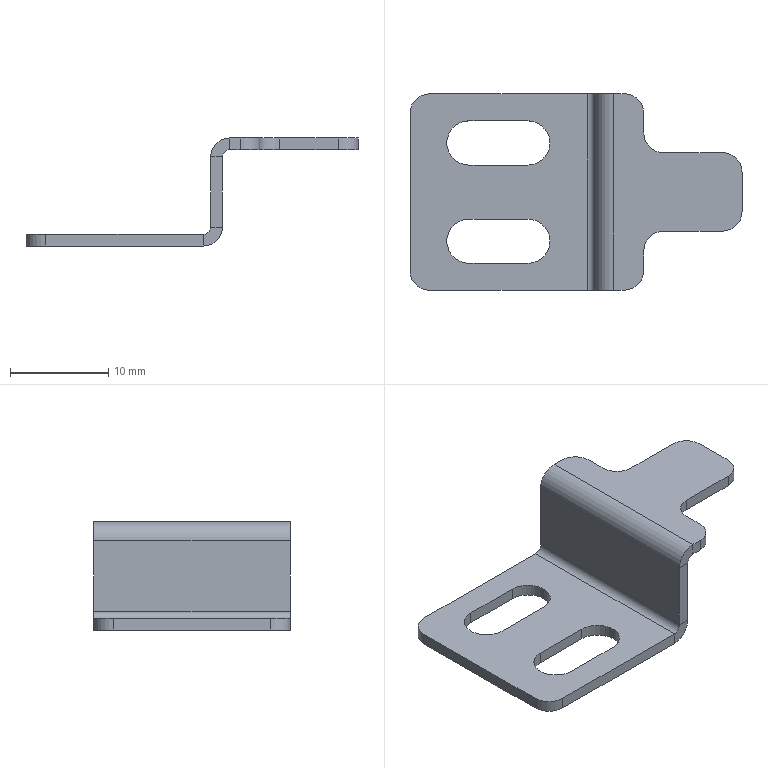Part | SolidWorks | features EdgeFlange 2, ICE 2, Fillet 1, FlatPattern 1, SMBaseFlange 1, SheetMetal 1 | 1 solid | 44 faces | box 33.8 x 20 x 11 mm | volume 767.773 mm3 | plane 26 | cylinder 18 | commonest cylinder face diameters 4 x8 4.5 x6 1.473 x2 3.873 x2
STEP:
#1=CARTESIAN_POINT('',(4.25,-5.,-1.2));
#2=VERTEX_POINT('',#1);
#3=CARTESIAN_POINT('',(2.,-2.75,-1.2));
#4=VERTEX_POINT('',#3);
#5=CARTESIAN_POINT('',(2.,-5.,-1.2));
#6=DIRECTION('',(0.,0.,1.));
#7=DIRECTION('',(-1.,0.,0.));
#8=AXIS2_PLACEMENT_3D('',#5,#6,#7);
#9=CIRCLE('',#8,2.25);
#10=EDGE_CURVE('',#2,#4,#9,.T.);
#11=ORIENTED_EDGE('',*,*,#10,.F.);
#12=CARTESIAN_POINT('',(4.25,-5.,0.));
#13=VERTEX_POINT('',#12);
#14=CARTESIAN_POINT('',(4.25,-5.,-1.2));
#15=DIRECTION('',(0.,0.,1.));
#16=VECTOR('',#15,1000.);
#17=LINE('',#14,#16);
#18=EDGE_CURVE('',#2,#13,#17,.T.);
#19=ORIENTED_EDGE('',*,*,#18,.T.);
#20=CARTESIAN_POINT('',(2.,-2.75,0.));
#21=VERTEX_POINT('',#20);
#22=CARTESIAN_POINT('',(2.,-5.,0.));
#23=DIRECTION('',(0.,0.,1.));
#24=DIRECTION('',(-1.,0.,0.));
#25=AXIS2_PLACEMENT_3D('',#22,#23,#24);
#26=CIRCLE('',#25,2.25);
#27=EDGE_CURVE('',#13,#21,#26,.T.);
#28=ORIENTED_EDGE('',*,*,#27,.T.);
#29=CARTESIAN_POINT('',(2.,-2.75,-1.2));
#30=DIRECTION('',(0.,0.,1.));
#31=VECTOR('',#30,1000.);
#32=LINE('',#29,#31);
#33=EDGE_CURVE('',#4,#21,#32,.T.);
#34=ORIENTED_EDGE('',*,*,#33,.F.);
#35=EDGE_LOOP('',(#11,#19,#28,#34));
#36=FACE_OUTER_BOUND('',#35,.T.);
#37=CARTESIAN_POINT('',(2.,-5.,-1.2));
#38=DIRECTION('',(0.,0.,1.));
#39=DIRECTION('',(1.,0.,0.));
#40=AXIS2_PLACEMENT_3D('',#37,#38,#39);
#41=CYLINDRICAL_SURFACE('',#40,2.25);
#42=ADVANCED_FACE('',(#36),#41,.F.);
#43=CARTESIAN_POINT('',(4.25,5.,-1.2));
#44=VERTEX_POINT('',#43);
#45=CARTESIAN_POINT('',(2.,7.25,-1.2));
#46=VERTEX_POINT('',#45);
#47=CARTESIAN_POINT('',(2.,5.,-1.2));
#48=DIRECTION('',(0.,0.,1.));
#49=DIRECTION('',(1.,0.,0.));
#50=AXIS2_PLACEMENT_3D('',#47,#48,#49);
#51=CIRCLE('',#50,2.25);
#52=EDGE_CURVE('',#44,#46,#51,.T.);
#53=ORIENTED_EDGE('',*,*,#52,.F.);
#54=CARTESIAN_POINT('',(4.25,5.,0.));
#55=VERTEX_POINT('',#54);
#56=CARTESIAN_POINT('',(4.25,5.,-1.2));
#57=DIRECTION('',(0.,0.,1.));
#58=VECTOR('',#57,1000.);
#59=LINE('',#56,#58);
#60=EDGE_CURVE('',#44,#55,#59,.T.);
#61=ORIENTED_EDGE('',*,*,#60,.T.);
#62=CARTESIAN_POINT('',(2.,7.25,0.));
#63=VERTEX_POINT('',#62);
#64=CARTESIAN_POINT('',(2.,5.,0.));
#65=DIRECTION('',(0.,0.,1.));
#66=DIRECTION('',(1.,0.,0.));
#67=AXIS2_PLACEMENT_3D('',#64,#65,#66);
#68=CIRCLE('',#67,2.25);
#69=EDGE_CURVE('',#55,#63,#68,.T.);
#70=ORIENTED_EDGE('',*,*,#69,.T.);
#71=CARTESIAN_POINT('',(2.,7.25,-1.2));
#72=DIRECTION('',(0.,0.,1.));
#73=VECTOR('',#72,1000.);
#74=LINE('',#71,#73);
#75=EDGE_CURVE('',#46,#63,#74,.T.);
#76=ORIENTED_EDGE('',*,*,#75,.F.);
#77=EDGE_LOOP('',(#53,#61,#70,#76));
#78=FACE_OUTER_BOUND('',#77,.T.);
#79=CARTESIAN_POINT('',(2.,5.,-1.2));
#80=DIRECTION('',(0.,0.,1.));
#81=DIRECTION('',(1.,0.,0.));
#82=AXIS2_PLACEMENT_3D('',#79,#80,#81);
#83=CYLINDRICAL_SURFACE('',#82,2.25);
#84=ADVANCED_FACE('',(#78),#83,.F.);
#85=CARTESIAN_POINT('',(10.,-10.,0.7366));
#86=VERTEX_POINT('',#85);
#87=CARTESIAN_POINT('',(10.,-10.,7.863));
#88=VERTEX_POINT('',#87);
#89=CARTESIAN_POINT('',(10.,-10.,9.8));
#90=DIRECTION('',(0.,0.,1.));
#91=VECTOR('',#90,1000.);
#92=LINE('',#89,#91);
#93=EDGE_CURVE('',#86,#88,#92,.T.);
#94=ORIENTED_EDGE('',*,*,#93,.T.);
#95=CARTESIAN_POINT('',(8.8,-10.,7.863));
#96=VERTEX_POINT('',#95);
#97=CARTESIAN_POINT('',(10.,-10.,7.863));
#98=DIRECTION('',(-1.,0.,0.));
#99=VECTOR('',#98,1000.);
#100=LINE('',#97,#99);
#101=EDGE_CURVE('',#88,#96,#100,.T.);
#102=ORIENTED_EDGE('',*,*,#101,.T.);
#103=CARTESIAN_POINT('',(8.8,-10.,0.7366));
#104=VERTEX_POINT('',#103);
#105=CARTESIAN_POINT('',(8.8,-10.,0.));
#106=DIRECTION('',(0.,0.,1.));
#107=VECTOR('',#106,1000.);
#108=LINE('',#105,#107);
#109=EDGE_CURVE('',#104,#96,#108,.T.);
#110=ORIENTED_EDGE('',*,*,#109,.F.);
#111=CARTESIAN_POINT('',(10.,-10.,0.7366));
#112=DIRECTION('',(1.,0.,0.));
#113=VECTOR('',#112,1000.);
#114=LINE('',#111,#113);
#115=EDGE_CURVE('',#104,#86,#114,.T.);
#116=ORIENTED_EDGE('',*,*,#115,.T.);
#117=EDGE_LOOP('',(#94,#102,#110,#116));
#118=FACE_OUTER_BOUND('',#117,.T.);
#119=CARTESIAN_POINT('',(10.,-10.,9.8));
#120=DIRECTION('',(0.,-1.,0.));
#121=DIRECTION('',(0.,0.,-1.));
#122=AXIS2_PLACEMENT_3D('',#119,#120,#121);
#123=PLANE('',#122);
#124=ADVANCED_FACE('',(#118),#123,.T.);
#125=CARTESIAN_POINT('',(10.,10.,7.863));
#126=VERTEX_POINT('',#125);
#127=CARTESIAN_POINT('',(10.,10.,0.7366));
#128=VERTEX_POINT('',#127);
#129=CARTESIAN_POINT('',(10.,10.,0.));
#130=DIRECTION('',(0.,0.,-1.));
#131=VECTOR('',#130,1000.);
#132=LINE('',#129,#131);
#133=EDGE_CURVE('',#126,#128,#132,.T.);
#134=ORIENTED_EDGE('',*,*,#133,.F.);
#135=CARTESIAN_POINT('',(10.,-10.,7.863));
#136=DIRECTION('',(0.,1.,0.));
#137=VECTOR('',#136,1000.);
#138=LINE('',#135,#137);
#139=EDGE_CURVE('',#88,#126,#138,.T.);
#140=ORIENTED_EDGE('',*,*,#139,.F.);
#141=ORIENTED_EDGE('',*,*,#93,.F.);
#142=CARTESIAN_POINT('',(10.,0.,0.7366));
#143=DIRECTION('',(0.,1.,0.));
#144=VECTOR('',#143,1000.);
#145=LINE('',#142,#144);
#146=EDGE_CURVE('',#86,#128,#145,.T.);
#147=ORIENTED_EDGE('',*,*,#146,.T.);
#148=EDGE_LOOP('',(#134,#140,#141,#147));
#149=FACE_OUTER_BOUND('',#148,.T.);
#150=CARTESIAN_POINT('',(10.,0.,0.));
#151=DIRECTION('',(1.,0.,0.));
#152=DIRECTION('',(0.,0.,-1.));
#153=AXIS2_PLACEMENT_3D('',#150,#151,#152);
#154=PLANE('',#153);
#155=ADVANCED_FACE('',(#149),#154,.T.);
#156=CARTESIAN_POINT('',(8.8,10.,7.863));
#157=VERTEX_POINT('',#156);
#158=CARTESIAN_POINT('',(8.8,-10.,7.863));
#159=DIRECTION('',(0.,1.,0.));
#160=VECTOR('',#159,1000.);
#161=LINE('',#158,#160);
#162=EDGE_CURVE('',#96,#157,#161,.T.);
#163=ORIENTED_EDGE('',*,*,#162,.T.);
#164=CARTESIAN_POINT('',(8.8,10.,0.7366));
#165=VERTEX_POINT('',#164);
#166=CARTESIAN_POINT('',(8.8,10.,0.));
#167=DIRECTION('',(0.,0.,-1.));
#168=VECTOR('',#167,1000.);
#169=LINE('',#166,#168);
#170=EDGE_CURVE('',#157,#165,#169,.T.);
#171=ORIENTED_EDGE('',*,*,#170,.T.);
#172=CARTESIAN_POINT('',(8.8,-10.,0.7366));
#173=DIRECTION('',(0.,1.,0.));
#174=VECTOR('',#173,1000.);
#175=LINE('',#172,#174);
#176=EDGE_CURVE('',#104,#165,#175,.T.);
#177=ORIENTED_EDGE('',*,*,#176,.F.);
#178=ORIENTED_EDGE('',*,*,#109,.T.);
#179=EDGE_LOOP('',(#163,#171,#177,#178));
#180=FACE_OUTER_BOUND('',#179,.T.);
#181=CARTESIAN_POINT('',(8.8,0.,0.));
#182=DIRECTION('',(1.,0.,0.));
#183=DIRECTION('',(0.,0.,-1.));
#184=AXIS2_PLACEMENT_3D('',#181,#182,#183);
#185=PLANE('',#184);
#186=ADVANCED_FACE('',(#180),#185,.F.);
#187=CARTESIAN_POINT('',(8.063,10.,-1.2));
#188=VERTEX_POINT('',#187);
#189=CARTESIAN_POINT('',(-8.,10.,-1.2));
#190=VERTEX_POINT('',#189);
#191=CARTESIAN_POINT('',(-10.,10.,-1.2));
#192=DIRECTION('',(-1.,0.,0.));
#193=VECTOR('',#192,1000.);
#194=LINE('',#191,#193);
#195=EDGE_CURVE('',#188,#190,#194,.T.);
#196=ORIENTED_EDGE('',*,*,#195,.T.);
#197=CARTESIAN_POINT('',(-8.,10.,0.));
#198=VERTEX_POINT('',#197);
#199=CARTESIAN_POINT('',(-8.,10.,-1.2));
#200=DIRECTION('',(0.,0.,1.));
#201=VECTOR('',#200,1000.);
#202=LINE('',#199,#201);
#203=EDGE_CURVE('',#190,#198,#202,.T.);
#204=ORIENTED_EDGE('',*,*,#203,.T.);
#205=CARTESIAN_POINT('',(8.063,10.,0.));
#206=VERTEX_POINT('',#205);
#207=CARTESIAN_POINT('',(-10.,10.,0.));
#208=DIRECTION('',(-1.,0.,0.));
#209=VECTOR('',#208,1000.);
#210=LINE('',#207,#209);
#211=EDGE_CURVE('',#206,#198,#210,.T.);
#212=ORIENTED_EDGE('',*,*,#211,.F.);
#213=CARTESIAN_POINT('',(8.063,10.,0.));
#214=DIRECTION('',(0.,0.,-1.));
#215=VECTOR('',#214,1000.);
#216=LINE('',#213,#215);
#217=EDGE_CURVE('',#206,#188,#216,.T.);
#218=ORIENTED_EDGE('',*,*,#217,.T.);
#219=EDGE_LOOP('',(#196,#204,#212,#218));
#220=FACE_OUTER_BOUND('',#219,.T.);
#221=CARTESIAN_POINT('',(-10.,10.,-1.2));
#222=DIRECTION('',(0.,1.,0.));
#223=DIRECTION('',(0.,0.,1.));
#224=AXIS2_PLACEMENT_3D('',#221,#222,#223);
#225=PLANE('',#224);
#226=ADVANCED_FACE('',(#220),#225,.T.);
#227=CARTESIAN_POINT('',(-4.,-2.75,-1.2));
#228=VERTEX_POINT('',#227);
#229=CARTESIAN_POINT('',(-4.,-7.25,-1.2));
#230=VERTEX_POINT('',#229);
#231=CARTESIAN_POINT('',(-4.,-5.,-1.2));
#232=DIRECTION('',(0.,0.,1.));
#233=DIRECTION('',(-1.,0.,0.));
#234=AXIS2_PLACEMENT_3D('',#231,#232,#233);
#235=CIRCLE('',#234,2.25);
#236=EDGE_CURVE('',#228,#230,#235,.T.);
#237=ORIENTED_EDGE('',*,*,#236,.T.);
#238=CARTESIAN_POINT('',(2.,-7.25,-1.2));
#239=VERTEX_POINT('',#238);
#240=CARTESIAN_POINT('',(-4.,-7.25,-1.2));
#241=DIRECTION('',(1.,0.,0.));
#242=VECTOR('',#241,1000.);
#243=LINE('',#240,#242);
#244=EDGE_CURVE('',#230,#239,#243,.T.);
#245=ORIENTED_EDGE('',*,*,#244,.T.);
#246=CARTESIAN_POINT('',(2.,-5.,-1.2));
#247=DIRECTION('',(0.,0.,1.));
#248=DIRECTION('',(-1.,0.,0.));
#249=AXIS2_PLACEMENT_3D('',#246,#247,#248);
#250=CIRCLE('',#249,2.25);
#251=EDGE_CURVE('',#239,#2,#250,.T.);
#252=ORIENTED_EDGE('',*,*,#251,.T.);
#253=ORIENTED_EDGE('',*,*,#10,.T.);
#254=CARTESIAN_POINT('',(-4.,-2.75,-1.2));
#255=DIRECTION('',(-1.,0.,0.));
#256=VECTOR('',#255,1000.);
#257=LINE('',#254,#256);
#258=EDGE_CURVE('',#4,#228,#257,.T.);
#259=ORIENTED_EDGE('',*,*,#258,.T.);
#260=EDGE_LOOP('',(#237,#245,#252,#253,#259));
#261=FACE_BOUND('',#260,.T.);
#262=CARTESIAN_POINT('',(-4.,7.25,-1.2));
#263=VERTEX_POINT('',#262);
#264=CARTESIAN_POINT('',(-4.,2.75,-1.2));
#265=VERTEX_POINT('',#264);
#266=CARTESIAN_POINT('',(-4.,5.,-1.2));
#267=DIRECTION('',(0.,0.,1.));
#268=DIRECTION('',(1.,0.,0.));
#269=AXIS2_PLACEMENT_3D('',#266,#267,#268);
#270=CIRCLE('',#269,2.25);
#271=EDGE_CURVE('',#263,#265,#270,.T.);
#272=ORIENTED_EDGE('',*,*,#271,.T.);
#273=CARTESIAN_POINT('',(2.,2.75,-1.2));
#274=VERTEX_POINT('',#273);
#275=CARTESIAN_POINT('',(-4.,2.75,-1.2));
#276=DIRECTION('',(1.,0.,0.));
#277=VECTOR('',#276,1000.);
#278=LINE('',#275,#277);
#279=EDGE_CURVE('',#265,#274,#278,.T.);
#280=ORIENTED_EDGE('',*,*,#279,.T.);
#281=CARTESIAN_POINT('',(2.,5.,-1.2));
#282=DIRECTION('',(0.,0.,1.));
#283=DIRECTION('',(1.,0.,0.));
#284=AXIS2_PLACEMENT_3D('',#281,#282,#283);
#285=CIRCLE('',#284,2.25);
#286=EDGE_CURVE('',#274,#44,#285,.T.);
#287=ORIENTED_EDGE('',*,*,#286,.T.);
#288=ORIENTED_EDGE('',*,*,#52,.T.);
#289=CARTESIAN_POINT('',(-4.,7.25,-1.2));
#290=DIRECTION('',(-1.,0.,0.));
#291=VECTOR('',#290,1000.);
#292=LINE('',#289,#291);
#293=EDGE_CURVE('',#46,#263,#292,.T.);
#294=ORIENTED_EDGE('',*,*,#293,.T.);
#295=EDGE_LOOP('',(#272,#280,#287,#288,#294));
#296=FACE_BOUND('',#295,.T.);
#297=CARTESIAN_POINT('',(-8.,-10.,-1.2));
#298=VERTEX_POINT('',#297);
#299=CARTESIAN_POINT('',(8.063,-10.,-1.2));
#300=VERTEX_POINT('',#299);
#301=CARTESIAN_POINT('',(-10.,-10.,-1.2));
#302=DIRECTION('',(1.,0.,0.));
#303=VECTOR('',#302,1000.);
#304=LINE('',#301,#303);
#305=EDGE_CURVE('',#298,#300,#304,.T.);
#306=ORIENTED_EDGE('',*,*,#305,.F.);
#307=CARTESIAN_POINT('',(-10.,-8.,-1.2));
#308=VERTEX_POINT('',#307);
#309=CARTESIAN_POINT('',(-8.,-8.,-1.2));
#310=DIRECTION('',(0.,0.,-1.));
#311=DIRECTION('',(-1.,0.,0.));
#312=AXIS2_PLACEMENT_3D('',#309,#310,#311);
#313=CIRCLE('',#312,2.);
#314=EDGE_CURVE('',#298,#308,#313,.T.);
#315=ORIENTED_EDGE('',*,*,#314,.T.);
#316=CARTESIAN_POINT('',(-10.,8.,-1.2));
#317=VERTEX_POINT('',#316);
#318=CARTESIAN_POINT('',(-10.,-10.,-1.2));
#319=DIRECTION('',(0.,-1.,0.));
#320=VECTOR('',#319,1000.);
#321=LINE('',#318,#320);
#322=EDGE_CURVE('',#317,#308,#321,.T.);
#323=ORIENTED_EDGE('',*,*,#322,.F.);
#324=CARTESIAN_POINT('',(-8.,8.,-1.2));
#325=DIRECTION('',(0.,0.,-1.));
#326=DIRECTION('',(-1.,0.,0.));
#327=AXIS2_PLACEMENT_3D('',#324,#325,#326);
#328=CIRCLE('',#327,2.);
#329=EDGE_CURVE('',#317,#190,#328,.T.);
#330=ORIENTED_EDGE('',*,*,#329,.T.);
#331=ORIENTED_EDGE('',*,*,#195,.F.);
#332=CARTESIAN_POINT('',(8.063,10.,-1.2));
#333=DIRECTION('',(0.,-1.,0.));
#334=VECTOR('',#333,1000.);
#335=LINE('',#332,#334);
#336=EDGE_CURVE('',#188,#300,#335,.T.);
#337=ORIENTED_EDGE('',*,*,#336,.T.);
#338=EDGE_LOOP('',(#306,#315,#323,#330,#331,#337));
#339=FACE_OUTER_BOUND('',#338,.T.);
#340=CARTESIAN_POINT('',(0.,0.,-1.2));
#341=DIRECTION('',(0.,0.,-1.));
#342=DIRECTION('',(-1.,0.,0.));
#343=AXIS2_PLACEMENT_3D('',#340,#341,#342);
#344=PLANE('',#343);
#345=ADVANCED_FACE('',(#261,#296,#339),#344,.T.);
#346=CARTESIAN_POINT('',(-4.,-7.25,0.));
#347=VERTEX_POINT('',#346);
#348=CARTESIAN_POINT('',(2.,-7.25,0.));
#349=VERTEX_POINT('',#348);
#350=CARTESIAN_POINT('',(-4.,-7.25,0.));
#351=DIRECTION('',(1.,0.,0.));
#352=VECTOR('',#351,1000.);
#353=LINE('',#350,#352);
#354=EDGE_CURVE('',#347,#349,#353,.T.);
#355=ORIENTED_EDGE('',*,*,#354,.F.);
#356=CARTESIAN_POINT('',(-4.,-2.75,0.));
#357=VERTEX_POINT('',#356);
#358=CARTESIAN_POINT('',(-4.,-5.,0.));
#359=DIRECTION('',(0.,0.,1.));
#360=DIRECTION('',(-1.,0.,0.));
#361=AXIS2_PLACEMENT_3D('',#358,#359,#360);
#362=CIRCLE('',#361,2.25);
#363=EDGE_CURVE('',#357,#347,#362,.T.);
#364=ORIENTED_EDGE('',*,*,#363,.F.);
#365=CARTESIAN_POINT('',(-4.,-2.75,0.));
#366=DIRECTION('',(-1.,0.,0.));
#367=VECTOR('',#366,1000.);
#368=LINE('',#365,#367);
#369=EDGE_CURVE('',#21,#357,#368,.T.);
#370=ORIENTED_EDGE('',*,*,#369,.F.);
#371=ORIENTED_EDGE('',*,*,#27,.F.);
#372=CARTESIAN_POINT('',(2.,-5.,0.));
#373=DIRECTION('',(0.,0.,1.));
#374=DIRECTION('',(-1.,0.,0.));
#375=AXIS2_PLACEMENT_3D('',#372,#373,#374);
#376=CIRCLE('',#375,2.25);
#377=EDGE_CURVE('',#349,#13,#376,.T.);
#378=ORIENTED_EDGE('',*,*,#377,.F.);
#379=EDGE_LOOP('',(#355,#364,#370,#371,#378));
#380=FACE_BOUND('',#379,.T.);
#381=CARTESIAN_POINT('',(-4.,2.75,0.));
#382=VERTEX_POINT('',#381);
#383=CARTESIAN_POINT('',(2.,2.75,0.));
#384=VERTEX_POINT('',#383);
#385=CARTESIAN_POINT('',(-4.,2.75,0.));
#386=DIRECTION('',(1.,0.,0.));
#387=VECTOR('',#386,1000.);
#388=LINE('',#385,#387);
#389=EDGE_CURVE('',#382,#384,#388,.T.);
#390=ORIENTED_EDGE('',*,*,#389,.F.);
#391=CARTESIAN_POINT('',(-4.,7.25,0.));
#392=VERTEX_POINT('',#391);
#393=CARTESIAN_POINT('',(-4.,5.,0.));
#394=DIRECTION('',(0.,0.,1.));
#395=DIRECTION('',(1.,0.,0.));
#396=AXIS2_PLACEMENT_3D('',#393,#394,#395);
#397=CIRCLE('',#396,2.25);
#398=EDGE_CURVE('',#392,#382,#397,.T.);
#399=ORIENTED_EDGE('',*,*,#398,.F.);
#400=CARTESIAN_POINT('',(-4.,7.25,0.));
#401=DIRECTION('',(-1.,0.,0.));
#402=VECTOR('',#401,1000.);
#403=LINE('',#400,#402);
#404=EDGE_CURVE('',#63,#392,#403,.T.);
#405=ORIENTED_EDGE('',*,*,#404,.F.);
#406=ORIENTED_EDGE('',*,*,#69,.F.);
#407=CARTESIAN_POINT('',(2.,5.,0.));
#408=DIRECTION('',(0.,0.,1.));
#409=DIRECTION('',(1.,0.,0.));
#410=AXIS2_PLACEMENT_3D('',#407,#408,#409);
#411=CIRCLE('',#410,2.25);
#412=EDGE_CURVE('',#384,#55,#411,.T.);
#413=ORIENTED_EDGE('',*,*,#412,.F.);
#414=EDGE_LOOP('',(#390,#399,#405,#406,#413));
#415=FACE_BOUND('',#414,.T.);
#416=CARTESIAN_POINT('',(-10.,8.,0.));
#417=VERTEX_POINT('',#416);
#418=CARTESIAN_POINT('',(-10.,-8.,0.));
#419=VERTEX_POINT('',#418);
#420=CARTESIAN_POINT('',(-10.,-10.,0.));
#421=DIRECTION('',(0.,-1.,0.));
#422=VECTOR('',#421,1000.);
#423=LINE('',#420,#422);
#424=EDGE_CURVE('',#417,#419,#423,.T.);
#425=ORIENTED_EDGE('',*,*,#424,.T.);
#426=CARTESIAN_POINT('',(-8.,-10.,0.));
#427=VERTEX_POINT('',#426);
#428=CARTESIAN_POINT('',(-8.,-8.,0.));
#429=DIRECTION('',(0.,0.,1.));
#430=DIRECTION('',(-1.,0.,0.));
#431=AXIS2_PLACEMENT_3D('',#428,#429,#430);
#432=CIRCLE('',#431,2.);
#433=EDGE_CURVE('',#419,#427,#432,.T.);
#434=ORIENTED_EDGE('',*,*,#433,.T.);
#435=CARTESIAN_POINT('',(8.063,-10.,0.));
#436=VERTEX_POINT('',#435);
#437=CARTESIAN_POINT('',(-10.,-10.,0.));
#438=DIRECTION('',(1.,0.,0.));
#439=VECTOR('',#438,1000.);
#440=LINE('',#437,#439);
#441=EDGE_CURVE('',#427,#436,#440,.T.);
#442=ORIENTED_EDGE('',*,*,#441,.T.);
#443=CARTESIAN_POINT('',(8.063,10.,0.));
#444=DIRECTION('',(0.,-1.,0.));
#445=VECTOR('',#444,1000.);
#446=LINE('',#443,#445);
#447=EDGE_CURVE('',#206,#436,#446,.T.);
#448=ORIENTED_EDGE('',*,*,#447,.F.);
#449=ORIENTED_EDGE('',*,*,#211,.T.);
#450=CARTESIAN_POINT('',(-8.,8.,0.));
#451=DIRECTION('',(0.,0.,1.));
#452=DIRECTION('',(-1.,0.,0.));
#453=AXIS2_PLACEMENT_3D('',#450,#451,#452);
#454=CIRCLE('',#453,2.);
#455=EDGE_CURVE('',#198,#417,#454,.T.);
#456=ORIENTED_EDGE('',*,*,#455,.T.);
#457=EDGE_LOOP('',(#425,#434,#442,#448,#449,#456));
#458=FACE_OUTER_BOUND('',#457,.T.);
#459=CARTESIAN_POINT('',(0.,0.,0.));
#460=DIRECTION('',(0.,0.,-1.));
#461=DIRECTION('',(-1.,0.,0.));
#462=AXIS2_PLACEMENT_3D('',#459,#460,#461);
#463=PLANE('',#462);
#464=ADVANCED_FACE('',(#380,#415,#458),#463,.F.);
#465=ORIENTED_EDGE('',*,*,#441,.F.);
#466=CARTESIAN_POINT('',(-8.,-10.,-1.2));
#467=DIRECTION('',(0.,0.,-1.));
#468=VECTOR('',#467,1000.);
#469=LINE('',#466,#468);
#470=EDGE_CURVE('',#427,#298,#469,.T.);
#471=ORIENTED_EDGE('',*,*,#470,.T.);
#472=ORIENTED_EDGE('',*,*,#305,.T.);
#473=CARTESIAN_POINT('',(8.063,-10.,0.));
#474=DIRECTION('',(0.,0.,-1.));
#475=VECTOR('',#474,1000.);
#476=LINE('',#473,#475);
#477=EDGE_CURVE('',#436,#300,#476,.T.);
#478=ORIENTED_EDGE('',*,*,#477,.F.);
#479=EDGE_LOOP('',(#465,#471,#472,#478));
#480=FACE_OUTER_BOUND('',#479,.T.);
#481=CARTESIAN_POINT('',(-10.,-10.,-1.2));
#482=DIRECTION('',(0.,-1.,0.));
#483=DIRECTION('',(0.,0.,-1.));
#484=AXIS2_PLACEMENT_3D('',#481,#482,#483);
#485=PLANE('',#484);
#486=ADVANCED_FACE('',(#480),#485,.T.);
#487=ORIENTED_EDGE('',*,*,#322,.T.);
#488=CARTESIAN_POINT('',(-10.,-8.,-1.2));
#489=DIRECTION('',(0.,0.,1.));
#490=VECTOR('',#489,1000.);
#491=LINE('',#488,#490);
#492=EDGE_CURVE('',#308,#419,#491,.T.);
#493=ORIENTED_EDGE('',*,*,#492,.T.);
#494=ORIENTED_EDGE('',*,*,#424,.F.);
#495=CARTESIAN_POINT('',(-10.,8.,-1.2));
#496=DIRECTION('',(0.,0.,-1.));
#497=VECTOR('',#496,1000.);
#498=LINE('',#495,#497);
#499=EDGE_CURVE('',#417,#317,#498,.T.);
#500=ORIENTED_EDGE('',*,*,#499,.T.);
#501=EDGE_LOOP('',(#487,#493,#494,#500));
#502=FACE_OUTER_BOUND('',#501,.T.);
#503=CARTESIAN_POINT('',(-10.,-10.,-1.2));
#504=DIRECTION('',(-1.,0.,0.));
#505=DIRECTION('',(0.,0.,1.));
#506=AXIS2_PLACEMENT_3D('',#503,#504,#505);
#507=PLANE('',#506);
#508=ADVANCED_FACE('',(#502),#507,.T.);
#509=ORIENTED_EDGE('',*,*,#115,.F.);
#510=CARTESIAN_POINT('',(8.063,-10.,0.7366));
#511=DIRECTION('',(0.,-1.,0.));
#512=DIRECTION('',(0.,0.,1.));
#513=AXIS2_PLACEMENT_3D('',#510,#511,#512);
#514=CIRCLE('',#513,0.7366);
#515=EDGE_CURVE('',#436,#104,#514,.T.);
#516=ORIENTED_EDGE('',*,*,#515,.F.);
#517=ORIENTED_EDGE('',*,*,#477,.T.);
#518=CARTESIAN_POINT('',(8.063,-10.,0.7366));
#519=DIRECTION('',(0.,-1.,0.));
#520=DIRECTION('',(0.,0.,1.));
#521=AXIS2_PLACEMENT_3D('',#518,#519,#520);
#522=CIRCLE('',#521,1.937);
#523=EDGE_CURVE('',#300,#86,#522,.T.);
#524=ORIENTED_EDGE('',*,*,#523,.T.);
#525=EDGE_LOOP('',(#509,#516,#517,#524));
#526=FACE_OUTER_BOUND('',#525,.T.);
#527=CARTESIAN_POINT('',(8.063,-10.,0.7366));
#528=DIRECTION('',(0.,-1.,0.));
#529=DIRECTION('',(0.,0.,-1.));
#530=AXIS2_PLACEMENT_3D('',#527,#528,#529);
#531=PLANE('',#530);
#532=ADVANCED_FACE('',(#526),#531,.T.);
#533=CARTESIAN_POINT('',(8.063,10.,0.7366));
#534=DIRECTION('',(0.,1.,0.));
#535=DIRECTION('',(0.,0.,1.));
#536=AXIS2_PLACEMENT_3D('',#533,#534,#535);
#537=CIRCLE('',#536,0.7366);
#538=EDGE_CURVE('',#165,#206,#537,.T.);
#539=ORIENTED_EDGE('',*,*,#538,.F.);
#540=CARTESIAN_POINT('',(8.8,10.,0.7366));
#541=DIRECTION('',(1.,0.,0.));
#542=VECTOR('',#541,1000.);
#543=LINE('',#540,#542);
#544=EDGE_CURVE('',#165,#128,#543,.T.);
#545=ORIENTED_EDGE('',*,*,#544,.T.);
#546=CARTESIAN_POINT('',(8.063,10.,0.7366));
#547=DIRECTION('',(0.,1.,0.));
#548=DIRECTION('',(0.,0.,1.));
#549=AXIS2_PLACEMENT_3D('',#546,#547,#548);
#550=CIRCLE('',#549,1.937);
#551=EDGE_CURVE('',#128,#188,#550,.T.);
#552=ORIENTED_EDGE('',*,*,#551,.T.);
#553=ORIENTED_EDGE('',*,*,#217,.F.);
#554=EDGE_LOOP('',(#539,#545,#552,#553));
#555=FACE_OUTER_BOUND('',#554,.T.);
#556=CARTESIAN_POINT('',(8.063,10.,0.7366));
#557=DIRECTION('',(0.,-1.,0.));
#558=DIRECTION('',(0.,0.,-1.));
#559=AXIS2_PLACEMENT_3D('',#556,#557,#558);
#560=PLANE('',#559);
#561=ADVANCED_FACE('',(#555),#560,.F.);
#562=ORIENTED_EDGE('',*,*,#336,.F.);
#563=ORIENTED_EDGE('',*,*,#551,.F.);
#564=ORIENTED_EDGE('',*,*,#146,.F.);
#565=ORIENTED_EDGE('',*,*,#523,.F.);
#566=EDGE_LOOP('',(#562,#563,#564,#565));
#567=FACE_OUTER_BOUND('',#566,.T.);
#568=CARTESIAN_POINT('',(8.063,10.,0.7366));
#569=DIRECTION('',(0.,1.,0.));
#570=DIRECTION('',(1.,0.,0.));
#571=AXIS2_PLACEMENT_3D('',#568,#569,#570);
#572=CYLINDRICAL_SURFACE('',#571,1.937);
#573=ADVANCED_FACE('',(#567),#572,.T.);
#574=ORIENTED_EDGE('',*,*,#447,.T.);
#575=ORIENTED_EDGE('',*,*,#515,.T.);
#576=ORIENTED_EDGE('',*,*,#176,.T.);
#577=ORIENTED_EDGE('',*,*,#538,.T.);
#578=EDGE_LOOP('',(#574,#575,#576,#577));
#579=FACE_OUTER_BOUND('',#578,.T.);
#580=CARTESIAN_POINT('',(8.063,10.,0.7366));
#581=DIRECTION('',(0.,1.,0.));
#582=DIRECTION('',(1.,0.,0.));
#583=AXIS2_PLACEMENT_3D('',#580,#581,#582);
#584=CYLINDRICAL_SURFACE('',#583,0.7366);
#585=ADVANCED_FACE('',(#579),#584,.F.);
#586=CARTESIAN_POINT('',(10.,10.,7.863));
#587=DIRECTION('',(-1.,0.,0.));
#588=VECTOR('',#587,1000.);
#589=LINE('',#586,#588);
#590=EDGE_CURVE('',#126,#157,#589,.T.);
#591=ORIENTED_EDGE('',*,*,#590,.F.);
#592=ORIENTED_EDGE('',*,*,#133,.T.);
#593=ORIENTED_EDGE('',*,*,#544,.F.);
#594=ORIENTED_EDGE('',*,*,#170,.F.);
#595=EDGE_LOOP('',(#591,#592,#593,#594));
#596=FACE_OUTER_BOUND('',#595,.T.);
#597=CARTESIAN_POINT('',(10.,10.,0.));
#598=DIRECTION('',(0.,1.,0.));
#599=DIRECTION('',(0.,0.,1.));
#600=AXIS2_PLACEMENT_3D('',#597,#598,#599);
#601=PLANE('',#600);
#602=ADVANCED_FACE('',(#596),#601,.T.);
#603=CARTESIAN_POINT('',(10.737,10.,8.6));
#604=VERTEX_POINT('',#603);
#605=CARTESIAN_POINT('',(10.737,10.,9.8));
#606=VERTEX_POINT('',#605);
#607=CARTESIAN_POINT('',(10.737,10.,9.8));
#608=DIRECTION('',(0.,0.,1.));
#609=VECTOR('',#608,1000.);
#610=LINE('',#607,#609);
#611=EDGE_CURVE('',#604,#606,#610,.T.);
#612=ORIENTED_EDGE('',*,*,#611,.F.);
#613=CARTESIAN_POINT('',(10.737,10.,7.863));
#614=DIRECTION('',(0.,1.,0.));
#615=DIRECTION('',(0.,0.,-1.));
#616=AXIS2_PLACEMENT_3D('',#613,#614,#615);
#617=CIRCLE('',#616,0.7366);
#618=EDGE_CURVE('',#126,#604,#617,.T.);
#619=ORIENTED_EDGE('',*,*,#618,.F.);
#620=ORIENTED_EDGE('',*,*,#590,.T.);
#621=CARTESIAN_POINT('',(10.737,10.,7.863));
#622=DIRECTION('',(0.,1.,0.));
#623=DIRECTION('',(0.,0.,-1.));
#624=AXIS2_PLACEMENT_3D('',#621,#622,#623);
#625=CIRCLE('',#624,1.937);
#626=EDGE_CURVE('',#157,#606,#625,.T.);
#627=ORIENTED_EDGE('',*,*,#626,.T.);
#628=EDGE_LOOP('',(#612,#619,#620,#627));
#629=FACE_OUTER_BOUND('',#628,.T.);
#630=CARTESIAN_POINT('',(10.737,10.,7.863));
#631=DIRECTION('',(0.,1.,0.));
#632=DIRECTION('',(0.,0.,1.));
#633=AXIS2_PLACEMENT_3D('',#630,#631,#632);
#634=PLANE('',#633);
#635=ADVANCED_FACE('',(#629),#634,.T.);
#636=CARTESIAN_POINT('',(10.737,-10.,8.6));
#637=VERTEX_POINT('',#636);
#638=CARTESIAN_POINT('',(10.737,-10.,7.863));
#639=DIRECTION('',(0.,-1.,0.));
#640=DIRECTION('',(0.,0.,-1.));
#641=AXIS2_PLACEMENT_3D('',#638,#639,#640);
#642=CIRCLE('',#641,0.7366);
#643=EDGE_CURVE('',#637,#88,#642,.T.);
#644=ORIENTED_EDGE('',*,*,#643,.F.);
#645=CARTESIAN_POINT('',(10.737,-10.,9.8));
#646=VERTEX_POINT('',#645);
#647=CARTESIAN_POINT('',(10.737,-10.,8.6));
#648=DIRECTION('',(0.,0.,1.));
#649=VECTOR('',#648,1000.);
#650=LINE('',#647,#649);
#651=EDGE_CURVE('',#637,#646,#650,.T.);
#652=ORIENTED_EDGE('',*,*,#651,.T.);
#653=CARTESIAN_POINT('',(10.737,-10.,7.863));
#654=DIRECTION('',(0.,-1.,0.));
#655=DIRECTION('',(0.,0.,-1.));
#656=AXIS2_PLACEMENT_3D('',#653,#654,#655);
#657=CIRCLE('',#656,1.937);
#658=EDGE_CURVE('',#646,#96,#657,.T.);
#659=ORIENTED_EDGE('',*,*,#658,.T.);
#660=ORIENTED_EDGE('',*,*,#101,.F.);
#661=EDGE_LOOP('',(#644,#652,#659,#660));
#662=FACE_OUTER_BOUND('',#661,.T.);
#663=CARTESIAN_POINT('',(10.737,-10.,7.863));
#664=DIRECTION('',(0.,1.,0.));
#665=DIRECTION('',(0.,0.,1.));
#666=AXIS2_PLACEMENT_3D('',#663,#664,#665);
#667=PLANE('',#666);
#668=ADVANCED_FACE('',(#662),#667,.F.);
#669=ORIENTED_EDGE('',*,*,#162,.F.);
#670=ORIENTED_EDGE('',*,*,#658,.F.);
#671=CARTESIAN_POINT('',(10.737,0.,9.8));
#672=DIRECTION('',(0.,-1.,0.));
#673=VECTOR('',#672,1000.);
#674=LINE('',#671,#673);
#675=EDGE_CURVE('',#606,#646,#674,.T.);
#676=ORIENTED_EDGE('',*,*,#675,.F.);
#677=ORIENTED_EDGE('',*,*,#626,.F.);
#678=EDGE_LOOP('',(#669,#670,#676,#677));
#679=FACE_OUTER_BOUND('',#678,.T.);
#680=CARTESIAN_POINT('',(10.737,-10.,7.863));
#681=DIRECTION('',(0.,-1.,0.));
#682=DIRECTION('',(0.,0.,1.));
#683=AXIS2_PLACEMENT_3D('',#680,#681,#682);
#684=CYLINDRICAL_SURFACE('',#683,1.937);
#685=ADVANCED_FACE('',(#679),#684,.T.);
#686=ORIENTED_EDGE('',*,*,#139,.T.);
#687=ORIENTED_EDGE('',*,*,#618,.T.);
#688=CARTESIAN_POINT('',(10.737,10.,8.6));
#689=DIRECTION('',(0.,-1.,0.));
#690=VECTOR('',#689,1000.);
#691=LINE('',#688,#690);
#692=EDGE_CURVE('',#604,#637,#691,.T.);
#693=ORIENTED_EDGE('',*,*,#692,.T.);
#694=ORIENTED_EDGE('',*,*,#643,.T.);
#695=EDGE_LOOP('',(#686,#687,#693,#694));
#696=FACE_OUTER_BOUND('',#695,.T.);
#697=CARTESIAN_POINT('',(10.737,-10.,7.863));
#698=DIRECTION('',(0.,-1.,0.));
#699=DIRECTION('',(0.,0.,1.));
#700=AXIS2_PLACEMENT_3D('',#697,#698,#699);
#701=CYLINDRICAL_SURFACE('',#700,0.7366);
#702=ADVANCED_FACE('',(#696),#701,.F.);
#703=CARTESIAN_POINT('',(11.8,-10.,8.6));
#704=VERTEX_POINT('',#703);
#705=CARTESIAN_POINT('',(0.,-10.,8.6));
#706=DIRECTION('',(-1.,0.,0.));
#707=VECTOR('',#706,1000.);
#708=LINE('',#705,#707);
#709=EDGE_CURVE('',#704,#637,#708,.T.);
#710=ORIENTED_EDGE('',*,*,#709,.F.);
#711=CARTESIAN_POINT('',(11.8,-10.,9.8));
#712=VERTEX_POINT('',#711);
#713=CARTESIAN_POINT('',(11.8,-10.,9.8));
#714=DIRECTION('',(0.,0.,1.));
#715=VECTOR('',#714,1000.);
#716=LINE('',#713,#715);
#717=EDGE_CURVE('',#704,#712,#716,.T.);
#718=ORIENTED_EDGE('',*,*,#717,.T.);
#719=CARTESIAN_POINT('',(10.,-10.,9.8));
#720=DIRECTION('',(-1.,0.,0.));
#721=VECTOR('',#720,1000.);
#722=LINE('',#719,#721);
#723=EDGE_CURVE('',#712,#646,#722,.T.);
#724=ORIENTED_EDGE('',*,*,#723,.T.);
#725=ORIENTED_EDGE('',*,*,#651,.F.);
#726=EDGE_LOOP('',(#710,#718,#724,#725));
#727=FACE_OUTER_BOUND('',#726,.T.);
#728=CARTESIAN_POINT('',(10.,-10.,9.8));
#729=DIRECTION('',(0.,-1.,0.));
#730=DIRECTION('',(0.,0.,-1.));
#731=AXIS2_PLACEMENT_3D('',#728,#729,#730);
#732=PLANE('',#731);
#733=ADVANCED_FACE('',(#727),#732,.T.);
#734=CARTESIAN_POINT('',(11.8,10.,9.8));
#735=VERTEX_POINT('',#734);
#736=CARTESIAN_POINT('',(23.8,10.,9.8));
#737=DIRECTION('',(1.,0.,0.));
#738=VECTOR('',#737,1000.);
#739=LINE('',#736,#738);
#740=EDGE_CURVE('',#606,#735,#739,.T.);
#741=ORIENTED_EDGE('',*,*,#740,.T.);
#742=CARTESIAN_POINT('',(11.8,10.,8.6));
#743=VERTEX_POINT('',#742);
#744=CARTESIAN_POINT('',(11.8,10.,8.6));
#745=DIRECTION('',(0.,0.,-1.));
#746=VECTOR('',#745,1000.);
#747=LINE('',#744,#746);
#748=EDGE_CURVE('',#735,#743,#747,.T.);
#749=ORIENTED_EDGE('',*,*,#748,.T.);
#750=CARTESIAN_POINT('',(0.,10.,8.6));
#751=DIRECTION('',(1.,0.,0.));
#752=VECTOR('',#751,1000.);
#753=LINE('',#750,#752);
#754=EDGE_CURVE('',#604,#743,#753,.T.);
#755=ORIENTED_EDGE('',*,*,#754,.F.);
#756=ORIENTED_EDGE('',*,*,#611,.T.);
#757=EDGE_LOOP('',(#741,#749,#755,#756));
#758=FACE_OUTER_BOUND('',#757,.T.);
#759=CARTESIAN_POINT('',(23.8,10.,9.8));
#760=DIRECTION('',(0.,1.,0.));
#761=DIRECTION('',(0.,0.,1.));
#762=AXIS2_PLACEMENT_3D('',#759,#760,#761);
#763=PLANE('',#762);
#764=ADVANCED_FACE('',(#758),#763,.T.);
#765=CARTESIAN_POINT('',(13.8,6.,9.8));
#766=VERTEX_POINT('',#765);
#767=CARTESIAN_POINT('',(13.8,8.,9.8));
#768=VERTEX_POINT('',#767);
#769=CARTESIAN_POINT('',(13.8,10.,9.8));
#770=DIRECTION('',(0.,1.,0.));
#771=VECTOR('',#770,1000.);
#772=LINE('',#769,#771);
#773=EDGE_CURVE('',#766,#768,#772,.T.);
#774=ORIENTED_EDGE('',*,*,#773,.T.);
#775=CARTESIAN_POINT('',(11.8,8.,9.8));
#776=DIRECTION('',(0.,0.,1.));
#777=DIRECTION('',(1.,0.,0.));
#778=AXIS2_PLACEMENT_3D('',#775,#776,#777);
#779=CIRCLE('',#778,2.);
#780=EDGE_CURVE('',#768,#735,#779,.T.);
#781=ORIENTED_EDGE('',*,*,#780,.T.);
#782=ORIENTED_EDGE('',*,*,#740,.F.);
#783=ORIENTED_EDGE('',*,*,#675,.T.);
#784=ORIENTED_EDGE('',*,*,#723,.F.);
#785=CARTESIAN_POINT('',(13.8,-8.,9.8));
#786=VERTEX_POINT('',#785);
#787=CARTESIAN_POINT('',(11.8,-8.,9.8));
#788=DIRECTION('',(0.,0.,1.));
#789=DIRECTION('',(1.,0.,0.));
#790=AXIS2_PLACEMENT_3D('',#787,#788,#789);
#791=CIRCLE('',#790,2.);
#792=EDGE_CURVE('',#712,#786,#791,.T.);
#793=ORIENTED_EDGE('',*,*,#792,.T.);
#794=CARTESIAN_POINT('',(13.8,-6.,9.8));
#795=VERTEX_POINT('',#794);
#796=CARTESIAN_POINT('',(13.8,-10.,9.8));
#797=DIRECTION('',(0.,1.,0.));
#798=VECTOR('',#797,1000.);
#799=LINE('',#796,#798);
#800=EDGE_CURVE('',#786,#795,#799,.T.);
#801=ORIENTED_EDGE('',*,*,#800,.T.);
#802=CARTESIAN_POINT('',(15.8,-4.,9.8));
#803=VERTEX_POINT('',#802);
#804=CARTESIAN_POINT('',(15.8,-6.,9.8));
#805=DIRECTION('',(0.,0.,-1.));
#806=DIRECTION('',(1.,0.,0.));
#807=AXIS2_PLACEMENT_3D('',#804,#805,#806);
#808=CIRCLE('',#807,2.);
#809=EDGE_CURVE('',#795,#803,#808,.T.);
#810=ORIENTED_EDGE('',*,*,#809,.T.);
#811=CARTESIAN_POINT('',(21.8,-4.,9.8));
#812=VERTEX_POINT('',#811);
#813=CARTESIAN_POINT('',(23.8,-4.,9.8));
#814=DIRECTION('',(1.,0.,0.));
#815=VECTOR('',#814,1000.);
#816=LINE('',#813,#815);
#817=EDGE_CURVE('',#803,#812,#816,.T.);
#818=ORIENTED_EDGE('',*,*,#817,.T.);
#819=CARTESIAN_POINT('',(23.8,-2.,9.8));
#820=VERTEX_POINT('',#819);
#821=CARTESIAN_POINT('',(21.8,-2.,9.8));
#822=DIRECTION('',(0.,0.,1.));
#823=DIRECTION('',(1.,0.,0.));
#824=AXIS2_PLACEMENT_3D('',#821,#822,#823);
#825=CIRCLE('',#824,2.);
#826=EDGE_CURVE('',#812,#820,#825,.T.);
#827=ORIENTED_EDGE('',*,*,#826,.T.);
#828=CARTESIAN_POINT('',(23.8,2.,9.8));
#829=VERTEX_POINT('',#828);
#830=CARTESIAN_POINT('',(23.8,-10.,9.8));
#831=DIRECTION('',(0.,-1.,0.));
#832=VECTOR('',#831,1000.);
#833=LINE('',#830,#832);
#834=EDGE_CURVE('',#829,#820,#833,.T.);
#835=ORIENTED_EDGE('',*,*,#834,.F.);
#836=CARTESIAN_POINT('',(21.8,4.,9.8));
#837=VERTEX_POINT('',#836);
#838=CARTESIAN_POINT('',(21.8,2.,9.8));
#839=DIRECTION('',(0.,0.,1.));
#840=DIRECTION('',(1.,0.,0.));
#841=AXIS2_PLACEMENT_3D('',#838,#839,#840);
#842=CIRCLE('',#841,2.);
#843=EDGE_CURVE('',#829,#837,#842,.T.);
#844=ORIENTED_EDGE('',*,*,#843,.T.);
#845=CARTESIAN_POINT('',(15.8,4.,9.8));
#846=VERTEX_POINT('',#845);
#847=CARTESIAN_POINT('',(23.8,4.,9.8));
#848=DIRECTION('',(-1.,0.,0.));
#849=VECTOR('',#848,1000.);
#850=LINE('',#847,#849);
#851=EDGE_CURVE('',#837,#846,#850,.T.);
#852=ORIENTED_EDGE('',*,*,#851,.T.);
#853=CARTESIAN_POINT('',(15.8,6.,9.8));
#854=DIRECTION('',(0.,0.,-1.));
#855=DIRECTION('',(1.,0.,0.));
#856=AXIS2_PLACEMENT_3D('',#853,#854,#855);
#857=CIRCLE('',#856,2.);
#858=EDGE_CURVE('',#846,#766,#857,.T.);
#859=ORIENTED_EDGE('',*,*,#858,.T.);
#860=EDGE_LOOP('',(#774,#781,#782,#783,#784,#793,#801,#810,#818,#827,#835,#844,#852,#859));
#861=FACE_OUTER_BOUND('',#860,.T.);
#862=CARTESIAN_POINT('',(0.,0.,9.8));
#863=DIRECTION('',(0.,0.,1.));
#864=DIRECTION('',(1.,0.,0.));
#865=AXIS2_PLACEMENT_3D('',#862,#863,#864);
#866=PLANE('',#865);
#867=ADVANCED_FACE('',(#861),#866,.T.);
#868=ORIENTED_EDGE('',*,*,#754,.T.);
#869=CARTESIAN_POINT('',(13.8,8.,8.6));
#870=VERTEX_POINT('',#869);
#871=CARTESIAN_POINT('',(11.8,8.,8.6));
#872=DIRECTION('',(0.,0.,-1.));
#873=DIRECTION('',(1.,0.,0.));
#874=AXIS2_PLACEMENT_3D('',#871,#872,#873);
#875=CIRCLE('',#874,2.);
#876=EDGE_CURVE('',#743,#870,#875,.T.);
#877=ORIENTED_EDGE('',*,*,#876,.T.);
#878=CARTESIAN_POINT('',(13.8,6.,8.6));
#879=VERTEX_POINT('',#878);
#880=CARTESIAN_POINT('',(13.8,10.,8.6));
#881=DIRECTION('',(0.,1.,0.));
#882=VECTOR('',#881,1000.);
#883=LINE('',#880,#882);
#884=EDGE_CURVE('',#879,#870,#883,.T.);
#885=ORIENTED_EDGE('',*,*,#884,.F.);
#886=CARTESIAN_POINT('',(15.8,4.,8.6));
#887=VERTEX_POINT('',#886);
#888=CARTESIAN_POINT('',(15.8,6.,8.6));
#889=DIRECTION('',(0.,0.,1.));
#890=DIRECTION('',(1.,0.,0.));
#891=AXIS2_PLACEMENT_3D('',#888,#889,#890);
#892=CIRCLE('',#891,2.);
#893=EDGE_CURVE('',#879,#887,#892,.T.);
#894=ORIENTED_EDGE('',*,*,#893,.T.);
#895=CARTESIAN_POINT('',(21.8,4.,8.6));
#896=VERTEX_POINT('',#895);
#897=CARTESIAN_POINT('',(23.8,4.,8.6));
#898=DIRECTION('',(-1.,0.,0.));
#899=VECTOR('',#898,1000.);
#900=LINE('',#897,#899);
#901=EDGE_CURVE('',#896,#887,#900,.T.);
#902=ORIENTED_EDGE('',*,*,#901,.F.);
#903=CARTESIAN_POINT('',(23.8,2.,8.6));
#904=VERTEX_POINT('',#903);
#905=CARTESIAN_POINT('',(21.8,2.,8.6));
#906=DIRECTION('',(0.,0.,-1.));
#907=DIRECTION('',(1.,0.,0.));
#908=AXIS2_PLACEMENT_3D('',#905,#906,#907);
#909=CIRCLE('',#908,2.);
#910=EDGE_CURVE('',#896,#904,#909,.T.);
#911=ORIENTED_EDGE('',*,*,#910,.T.);
#912=CARTESIAN_POINT('',(23.8,-2.,8.6));
#913=VERTEX_POINT('',#912);
#914=CARTESIAN_POINT('',(23.8,0.,8.6));
#915=DIRECTION('',(0.,-1.,0.));
#916=VECTOR('',#915,1000.);
#917=LINE('',#914,#916);
#918=EDGE_CURVE('',#904,#913,#917,.T.);
#919=ORIENTED_EDGE('',*,*,#918,.T.);
#920=CARTESIAN_POINT('',(21.8,-4.,8.6));
#921=VERTEX_POINT('',#920);
#922=CARTESIAN_POINT('',(21.8,-2.,8.6));
#923=DIRECTION('',(0.,0.,-1.));
#924=DIRECTION('',(1.,0.,0.));
#925=AXIS2_PLACEMENT_3D('',#922,#923,#924);
#926=CIRCLE('',#925,2.);
#927=EDGE_CURVE('',#913,#921,#926,.T.);
#928=ORIENTED_EDGE('',*,*,#927,.T.);
#929=CARTESIAN_POINT('',(15.8,-4.,8.6));
#930=VERTEX_POINT('',#929);
#931=CARTESIAN_POINT('',(23.8,-4.,8.6));
#932=DIRECTION('',(1.,0.,0.));
#933=VECTOR('',#932,1000.);
#934=LINE('',#931,#933);
#935=EDGE_CURVE('',#930,#921,#934,.T.);
#936=ORIENTED_EDGE('',*,*,#935,.F.);
#937=CARTESIAN_POINT('',(13.8,-6.,8.6));
#938=VERTEX_POINT('',#937);
#939=CARTESIAN_POINT('',(15.8,-6.,8.6));
#940=DIRECTION('',(0.,0.,1.));
#941=DIRECTION('',(1.,0.,0.));
#942=AXIS2_PLACEMENT_3D('',#939,#940,#941);
#943=CIRCLE('',#942,2.);
#944=EDGE_CURVE('',#930,#938,#943,.T.);
#945=ORIENTED_EDGE('',*,*,#944,.T.);
#946=CARTESIAN_POINT('',(13.8,-8.,8.6));
#947=VERTEX_POINT('',#946);
#948=CARTESIAN_POINT('',(13.8,-10.,8.6));
#949=DIRECTION('',(0.,1.,0.));
#950=VECTOR('',#949,1000.);
#951=LINE('',#948,#950);
#952=EDGE_CURVE('',#947,#938,#951,.T.);
#953=ORIENTED_EDGE('',*,*,#952,.F.);
#954=CARTESIAN_POINT('',(11.8,-8.,8.6));
#955=DIRECTION('',(0.,0.,-1.));
#956=DIRECTION('',(1.,0.,0.));
#957=AXIS2_PLACEMENT_3D('',#954,#955,#956);
#958=CIRCLE('',#957,2.);
#959=EDGE_CURVE('',#947,#704,#958,.T.);
#960=ORIENTED_EDGE('',*,*,#959,.T.);
#961=ORIENTED_EDGE('',*,*,#709,.T.);
#962=ORIENTED_EDGE('',*,*,#692,.F.);
#963=EDGE_LOOP('',(#868,#877,#885,#894,#902,#911,#919,#928,#936,#945,#953,#960,#961,#962));
#964=FACE_OUTER_BOUND('',#963,.T.);
#965=CARTESIAN_POINT('',(0.,0.,8.6));
#966=DIRECTION('',(0.,0.,1.));
#967=DIRECTION('',(1.,0.,0.));
#968=AXIS2_PLACEMENT_3D('',#965,#966,#967);
#969=PLANE('',#968);
#970=ADVANCED_FACE('',(#964),#969,.F.);
#971=ORIENTED_EDGE('',*,*,#834,.T.);
#972=CARTESIAN_POINT('',(23.8,-2.,8.6));
#973=DIRECTION('',(0.,0.,-1.));
#974=VECTOR('',#973,1000.);
#975=LINE('',#972,#974);
#976=EDGE_CURVE('',#820,#913,#975,.T.);
#977=ORIENTED_EDGE('',*,*,#976,.T.);
#978=ORIENTED_EDGE('',*,*,#918,.F.);
#979=CARTESIAN_POINT('',(23.8,2.,9.8));
#980=DIRECTION('',(0.,0.,1.));
#981=VECTOR('',#980,1000.);
#982=LINE('',#979,#981);
#983=EDGE_CURVE('',#904,#829,#982,.T.);
#984=ORIENTED_EDGE('',*,*,#983,.T.);
#985=EDGE_LOOP('',(#971,#977,#978,#984));
#986=FACE_OUTER_BOUND('',#985,.T.);
#987=CARTESIAN_POINT('',(23.8,-10.,9.8));
#988=DIRECTION('',(1.,0.,0.));
#989=DIRECTION('',(0.,0.,-1.));
#990=AXIS2_PLACEMENT_3D('',#987,#988,#989);
#991=PLANE('',#990);
#992=ADVANCED_FACE('',(#986),#991,.T.);
#993=ORIENTED_EDGE('',*,*,#884,.T.);
#994=CARTESIAN_POINT('',(13.8,8.,9.8));
#995=DIRECTION('',(0.,0.,1.));
#996=VECTOR('',#995,1000.);
#997=LINE('',#994,#996);
#998=EDGE_CURVE('',#870,#768,#997,.T.);
#999=ORIENTED_EDGE('',*,*,#998,.T.);
#1000=ORIENTED_EDGE('',*,*,#773,.F.);
#1001=CARTESIAN_POINT('',(13.8,6.,8.6));
#1002=DIRECTION('',(0.,0.,-1.));
#1003=VECTOR('',#1002,1000.);
#1004=LINE('',#1001,#1003);
#1005=EDGE_CURVE('',#766,#879,#1004,.T.);
#1006=ORIENTED_EDGE('',*,*,#1005,.T.);
#1007=EDGE_LOOP('',(#993,#999,#1000,#1006));
#1008=FACE_OUTER_BOUND('',#1007,.T.);
#1009=CARTESIAN_POINT('',(13.8,10.,9.8));
#1010=DIRECTION('',(-1.,0.,0.));
#1011=DIRECTION('',(0.,0.,1.));
#1012=AXIS2_PLACEMENT_3D('',#1009,#1010,#1011);
#1013=PLANE('',#1012);
#1014=ADVANCED_FACE('',(#1008),#1013,.F.);
#1015=ORIENTED_EDGE('',*,*,#901,.T.);
#1016=CARTESIAN_POINT('',(15.8,4.,9.8));
#1017=DIRECTION('',(0.,0.,1.));
#1018=VECTOR('',#1017,1000.);
#1019=LINE('',#1016,#1018);
#1020=EDGE_CURVE('',#887,#846,#1019,.T.);
#1021=ORIENTED_EDGE('',*,*,#1020,.T.);
#1022=ORIENTED_EDGE('',*,*,#851,.F.);
#1023=CARTESIAN_POINT('',(21.8,4.,8.6));
#1024=DIRECTION('',(0.,0.,-1.));
#1025=VECTOR('',#1024,1000.);
#1026=LINE('',#1023,#1025);
#1027=EDGE_CURVE('',#837,#896,#1026,.T.);
#1028=ORIENTED_EDGE('',*,*,#1027,.T.);
#1029=EDGE_LOOP('',(#1015,#1021,#1022,#1028));
#1030=FACE_OUTER_BOUND('',#1029,.T.);
#1031=CARTESIAN_POINT('',(23.8,4.,9.8));
#1032=DIRECTION('',(0.,-1.,0.));
#1033=DIRECTION('',(0.,0.,-1.));
#1034=AXIS2_PLACEMENT_3D('',#1031,#1032,#1033);
#1035=PLANE('',#1034);
#1036=ADVANCED_FACE('',(#1030),#1035,.F.);
#1037=ORIENTED_EDGE('',*,*,#817,.F.);
#1038=CARTESIAN_POINT('',(15.8,-4.,8.6));
#1039=DIRECTION('',(0.,0.,-1.));
#1040=VECTOR('',#1039,1000.);
#1041=LINE('',#1038,#1040);
#1042=EDGE_CURVE('',#803,#930,#1041,.T.);
#1043=ORIENTED_EDGE('',*,*,#1042,.T.);
#1044=ORIENTED_EDGE('',*,*,#935,.T.);
#1045=CARTESIAN_POINT('',(21.8,-4.,9.8));
#1046=DIRECTION('',(0.,0.,1.));
#1047=VECTOR('',#1046,1000.);
#1048=LINE('',#1045,#1047);
#1049=EDGE_CURVE('',#921,#812,#1048,.T.);
#1050=ORIENTED_EDGE('',*,*,#1049,.T.);
#1051=EDGE_LOOP('',(#1037,#1043,#1044,#1050));
#1052=FACE_OUTER_BOUND('',#1051,.T.);
#1053=CARTESIAN_POINT('',(23.8,-4.,9.8));
#1054=DIRECTION('',(0.,1.,0.));
#1055=DIRECTION('',(0.,0.,1.));
#1056=AXIS2_PLACEMENT_3D('',#1053,#1054,#1055);
#1057=PLANE('',#1056);
#1058=ADVANCED_FACE('',(#1052),#1057,.F.);
#1059=ORIENTED_EDGE('',*,*,#800,.F.);
#1060=CARTESIAN_POINT('',(13.8,-8.,8.6));
#1061=DIRECTION('',(0.,0.,-1.));
#1062=VECTOR('',#1061,1000.);
#1063=LINE('',#1060,#1062);
#1064=EDGE_CURVE('',#786,#947,#1063,.T.);
#1065=ORIENTED_EDGE('',*,*,#1064,.T.);
#1066=ORIENTED_EDGE('',*,*,#952,.T.);
#1067=CARTESIAN_POINT('',(13.8,-6.,9.8));
#1068=DIRECTION('',(0.,0.,1.));
#1069=VECTOR('',#1068,1000.);
#1070=LINE('',#1067,#1069);
#1071=EDGE_CURVE('',#938,#795,#1070,.T.);
#1072=ORIENTED_EDGE('',*,*,#1071,.T.);
#1073=EDGE_LOOP('',(#1059,#1065,#1066,#1072));
#1074=FACE_OUTER_BOUND('',#1073,.T.);
#1075=CARTESIAN_POINT('',(13.8,-10.,9.8));
#1076=DIRECTION('',(-1.,0.,0.));
#1077=DIRECTION('',(0.,0.,1.));
#1078=AXIS2_PLACEMENT_3D('',#1075,#1076,#1077);
#1079=PLANE('',#1078);
#1080=ADVANCED_FACE('',(#1074),#1079,.F.);
#1081=ORIENTED_EDGE('',*,*,#314,.F.);
#1082=ORIENTED_EDGE('',*,*,#470,.F.);
#1083=ORIENTED_EDGE('',*,*,#433,.F.);
#1084=ORIENTED_EDGE('',*,*,#492,.F.);
#1085=EDGE_LOOP('',(#1081,#1082,#1083,#1084));
#1086=FACE_OUTER_BOUND('',#1085,.T.);
#1087=CARTESIAN_POINT('',(-8.,-8.,-1.2));
#1088=DIRECTION('',(0.,0.,1.));
#1089=DIRECTION('',(1.,0.,0.));
#1090=AXIS2_PLACEMENT_3D('',#1087,#1088,#1089);
#1091=CYLINDRICAL_SURFACE('',#1090,2.);
#1092=ADVANCED_FACE('',(#1086),#1091,.T.);
#1093=ORIENTED_EDGE('',*,*,#329,.F.);
#1094=ORIENTED_EDGE('',*,*,#499,.F.);
#1095=ORIENTED_EDGE('',*,*,#455,.F.);
#1096=ORIENTED_EDGE('',*,*,#203,.F.);
#1097=EDGE_LOOP('',(#1093,#1094,#1095,#1096));
#1098=FACE_OUTER_BOUND('',#1097,.T.);
#1099=CARTESIAN_POINT('',(-8.,8.,-1.2));
#1100=DIRECTION('',(0.,0.,1.));
#1101=DIRECTION('',(1.,0.,0.));
#1102=AXIS2_PLACEMENT_3D('',#1099,#1100,#1101);
#1103=CYLINDRICAL_SURFACE('',#1102,2.);
#1104=ADVANCED_FACE('',(#1098),#1103,.T.);
#1105=ORIENTED_EDGE('',*,*,#780,.F.);
#1106=ORIENTED_EDGE('',*,*,#998,.F.);
#1107=ORIENTED_EDGE('',*,*,#876,.F.);
#1108=ORIENTED_EDGE('',*,*,#748,.F.);
#1109=EDGE_LOOP('',(#1105,#1106,#1107,#1108));
#1110=FACE_OUTER_BOUND('',#1109,.T.);
#1111=CARTESIAN_POINT('',(11.8,8.,9.8));
#1112=DIRECTION('',(0.,0.,1.));
#1113=DIRECTION('',(1.,0.,0.));
#1114=AXIS2_PLACEMENT_3D('',#1111,#1112,#1113);
#1115=CYLINDRICAL_SURFACE('',#1114,2.);
#1116=ADVANCED_FACE('',(#1110),#1115,.T.);
#1117=ORIENTED_EDGE('',*,*,#858,.F.);
#1118=ORIENTED_EDGE('',*,*,#1020,.F.);
#1119=ORIENTED_EDGE('',*,*,#893,.F.);
#1120=ORIENTED_EDGE('',*,*,#1005,.F.);
#1121=EDGE_LOOP('',(#1117,#1118,#1119,#1120));
#1122=FACE_OUTER_BOUND('',#1121,.T.);
#1123=CARTESIAN_POINT('',(15.8,6.,9.8));
#1124=DIRECTION('',(0.,0.,1.));
#1125=DIRECTION('',(1.,0.,0.));
#1126=AXIS2_PLACEMENT_3D('',#1123,#1124,#1125);
#1127=CYLINDRICAL_SURFACE('',#1126,2.);
#1128=ADVANCED_FACE('',(#1122),#1127,.F.);
#1129=ORIENTED_EDGE('',*,*,#792,.F.);
#1130=ORIENTED_EDGE('',*,*,#717,.F.);
#1131=ORIENTED_EDGE('',*,*,#959,.F.);
#1132=ORIENTED_EDGE('',*,*,#1064,.F.);
#1133=EDGE_LOOP('',(#1129,#1130,#1131,#1132));
#1134=FACE_OUTER_BOUND('',#1133,.T.);
#1135=CARTESIAN_POINT('',(11.8,-8.,9.8));
#1136=DIRECTION('',(0.,0.,1.));
#1137=DIRECTION('',(1.,0.,0.));
#1138=AXIS2_PLACEMENT_3D('',#1135,#1136,#1137);
#1139=CYLINDRICAL_SURFACE('',#1138,2.);
#1140=ADVANCED_FACE('',(#1134),#1139,.T.);
#1141=ORIENTED_EDGE('',*,*,#809,.F.);
#1142=ORIENTED_EDGE('',*,*,#1071,.F.);
#1143=ORIENTED_EDGE('',*,*,#944,.F.);
#1144=ORIENTED_EDGE('',*,*,#1042,.F.);
#1145=EDGE_LOOP('',(#1141,#1142,#1143,#1144));
#1146=FACE_OUTER_BOUND('',#1145,.T.);
#1147=CARTESIAN_POINT('',(15.8,-6.,9.8));
#1148=DIRECTION('',(0.,0.,1.));
#1149=DIRECTION('',(1.,0.,0.));
#1150=AXIS2_PLACEMENT_3D('',#1147,#1148,#1149);
#1151=CYLINDRICAL_SURFACE('',#1150,2.);
#1152=ADVANCED_FACE('',(#1146),#1151,.F.);
#1153=ORIENTED_EDGE('',*,*,#826,.F.);
#1154=ORIENTED_EDGE('',*,*,#1049,.F.);
#1155=ORIENTED_EDGE('',*,*,#927,.F.);
#1156=ORIENTED_EDGE('',*,*,#976,.F.);
#1157=EDGE_LOOP('',(#1153,#1154,#1155,#1156));
#1158=FACE_OUTER_BOUND('',#1157,.T.);
#1159=CARTESIAN_POINT('',(21.8,-2.,9.8));
#1160=DIRECTION('',(0.,0.,1.));
#1161=DIRECTION('',(1.,0.,0.));
#1162=AXIS2_PLACEMENT_3D('',#1159,#1160,#1161);
#1163=CYLINDRICAL_SURFACE('',#1162,2.);
#1164=ADVANCED_FACE('',(#1158),#1163,.T.);
#1165=ORIENTED_EDGE('',*,*,#843,.F.);
#1166=ORIENTED_EDGE('',*,*,#983,.F.);
#1167=ORIENTED_EDGE('',*,*,#910,.F.);
#1168=ORIENTED_EDGE('',*,*,#1027,.F.);
#1169=EDGE_LOOP('',(#1165,#1166,#1167,#1168));
#1170=FACE_OUTER_BOUND('',#1169,.T.);
#1171=CARTESIAN_POINT('',(21.8,2.,9.8));
#1172=DIRECTION('',(0.,0.,1.));
#1173=DIRECTION('',(1.,0.,0.));
#1174=AXIS2_PLACEMENT_3D('',#1171,#1172,#1173);
#1175=CYLINDRICAL_SURFACE('',#1174,2.);
#1176=ADVANCED_FACE('',(#1170),#1175,.T.);
#1177=ORIENTED_EDGE('',*,*,#398,.T.);
#1178=CARTESIAN_POINT('',(-4.,2.75,-1.2));
#1179=DIRECTION('',(0.,0.,1.));
#1180=VECTOR('',#1179,1000.);
#1181=LINE('',#1178,#1180);
#1182=EDGE_CURVE('',#265,#382,#1181,.T.);
#1183=ORIENTED_EDGE('',*,*,#1182,.F.);
#1184=ORIENTED_EDGE('',*,*,#271,.F.);
#1185=CARTESIAN_POINT('',(-4.,7.25,-1.2));
#1186=DIRECTION('',(0.,0.,1.));
#1187=VECTOR('',#1186,1000.);
#1188=LINE('',#1185,#1187);
#1189=EDGE_CURVE('',#263,#392,#1188,.T.);
#1190=ORIENTED_EDGE('',*,*,#1189,.T.);
#1191=EDGE_LOOP('',(#1177,#1183,#1184,#1190));
#1192=FACE_OUTER_BOUND('',#1191,.T.);
#1193=CARTESIAN_POINT('',(-4.,5.,-1.2));
#1194=DIRECTION('',(0.,0.,1.));
#1195=DIRECTION('',(1.,0.,0.));
#1196=AXIS2_PLACEMENT_3D('',#1193,#1194,#1195);
#1197=CYLINDRICAL_SURFACE('',#1196,2.25);
#1198=ADVANCED_FACE('',(#1192),#1197,.F.);
#1199=ORIENTED_EDGE('',*,*,#404,.T.);
#1200=ORIENTED_EDGE('',*,*,#1189,.F.);
#1201=ORIENTED_EDGE('',*,*,#293,.F.);
#1202=ORIENTED_EDGE('',*,*,#75,.T.);
#1203=EDGE_LOOP('',(#1199,#1200,#1201,#1202));
#1204=FACE_OUTER_BOUND('',#1203,.T.);
#1205=CARTESIAN_POINT('',(-4.,7.25,-1.2));
#1206=DIRECTION('',(0.,1.,0.));
#1207=DIRECTION('',(0.,0.,1.));
#1208=AXIS2_PLACEMENT_3D('',#1205,#1206,#1207);
#1209=PLANE('',#1208);
#1210=ADVANCED_FACE('',(#1204),#1209,.F.);
#1211=ORIENTED_EDGE('',*,*,#60,.F.);
#1212=ORIENTED_EDGE('',*,*,#286,.F.);
#1213=CARTESIAN_POINT('',(2.,2.75,-1.2));
#1214=DIRECTION('',(0.,0.,1.));
#1215=VECTOR('',#1214,1000.);
#1216=LINE('',#1213,#1215);
#1217=EDGE_CURVE('',#274,#384,#1216,.T.);
#1218=ORIENTED_EDGE('',*,*,#1217,.T.);
#1219=ORIENTED_EDGE('',*,*,#412,.T.);
#1220=EDGE_LOOP('',(#1211,#1212,#1218,#1219));
#1221=FACE_OUTER_BOUND('',#1220,.T.);
#1222=CARTESIAN_POINT('',(2.,5.,-1.2));
#1223=DIRECTION('',(0.,0.,1.));
#1224=DIRECTION('',(1.,0.,0.));
#1225=AXIS2_PLACEMENT_3D('',#1222,#1223,#1224);
#1226=CYLINDRICAL_SURFACE('',#1225,2.25);
#1227=ADVANCED_FACE('',(#1221),#1226,.F.);
#1228=ORIENTED_EDGE('',*,*,#389,.T.);
#1229=ORIENTED_EDGE('',*,*,#1217,.F.);
#1230=ORIENTED_EDGE('',*,*,#279,.F.);
#1231=ORIENTED_EDGE('',*,*,#1182,.T.);
#1232=EDGE_LOOP('',(#1228,#1229,#1230,#1231));
#1233=FACE_OUTER_BOUND('',#1232,.T.);
#1234=CARTESIAN_POINT('',(-4.,2.75,-1.2));
#1235=DIRECTION('',(0.,-1.,0.));
#1236=DIRECTION('',(0.,0.,-1.));
#1237=AXIS2_PLACEMENT_3D('',#1234,#1235,#1236);
#1238=PLANE('',#1237);
#1239=ADVANCED_FACE('',(#1233),#1238,.F.);
#1240=ORIENTED_EDGE('',*,*,#363,.T.);
#1241=CARTESIAN_POINT('',(-4.,-7.25,-1.2));
#1242=DIRECTION('',(0.,0.,1.));
#1243=VECTOR('',#1242,1000.);
#1244=LINE('',#1241,#1243);
#1245=EDGE_CURVE('',#230,#347,#1244,.T.);
#1246=ORIENTED_EDGE('',*,*,#1245,.F.);
#1247=ORIENTED_EDGE('',*,*,#236,.F.);
#1248=CARTESIAN_POINT('',(-4.,-2.75,-1.2));
#1249=DIRECTION('',(0.,0.,1.));
#1250=VECTOR('',#1249,1000.);
#1251=LINE('',#1248,#1250);
#1252=EDGE_CURVE('',#228,#357,#1251,.T.);
#1253=ORIENTED_EDGE('',*,*,#1252,.T.);
#1254=EDGE_LOOP('',(#1240,#1246,#1247,#1253));
#1255=FACE_OUTER_BOUND('',#1254,.T.);
#1256=CARTESIAN_POINT('',(-4.,-5.,-1.2));
#1257=DIRECTION('',(0.,0.,1.));
#1258=DIRECTION('',(1.,0.,0.));
#1259=AXIS2_PLACEMENT_3D('',#1256,#1257,#1258);
#1260=CYLINDRICAL_SURFACE('',#1259,2.25);
#1261=ADVANCED_FACE('',(#1255),#1260,.F.);
#1262=ORIENTED_EDGE('',*,*,#369,.T.);
#1263=ORIENTED_EDGE('',*,*,#1252,.F.);
#1264=ORIENTED_EDGE('',*,*,#258,.F.);
#1265=ORIENTED_EDGE('',*,*,#33,.T.);
#1266=EDGE_LOOP('',(#1262,#1263,#1264,#1265));
#1267=FACE_OUTER_BOUND('',#1266,.T.);
#1268=CARTESIAN_POINT('',(-4.,-2.75,-1.2));
#1269=DIRECTION('',(0.,1.,0.));
#1270=DIRECTION('',(-1.,0.,0.));
#1271=AXIS2_PLACEMENT_3D('',#1268,#1269,#1270);
#1272=PLANE('',#1271);
#1273=ADVANCED_FACE('',(#1267),#1272,.F.);
#1274=ORIENTED_EDGE('',*,*,#18,.F.);
#1275=ORIENTED_EDGE('',*,*,#251,.F.);
#1276=CARTESIAN_POINT('',(2.,-7.25,-1.2));
#1277=DIRECTION('',(0.,0.,1.));
#1278=VECTOR('',#1277,1000.);
#1279=LINE('',#1276,#1278);
#1280=EDGE_CURVE('',#239,#349,#1279,.T.);
#1281=ORIENTED_EDGE('',*,*,#1280,.T.);
#1282=ORIENTED_EDGE('',*,*,#377,.T.);
#1283=EDGE_LOOP('',(#1274,#1275,#1281,#1282));
#1284=FACE_OUTER_BOUND('',#1283,.T.);
#1285=CARTESIAN_POINT('',(2.,-5.,-1.2));
#1286=DIRECTION('',(0.,0.,1.));
#1287=DIRECTION('',(1.,0.,0.));
#1288=AXIS2_PLACEMENT_3D('',#1285,#1286,#1287);
#1289=CYLINDRICAL_SURFACE('',#1288,2.25);
#1290=ADVANCED_FACE('',(#1284),#1289,.F.);
#1291=ORIENTED_EDGE('',*,*,#354,.T.);
#1292=ORIENTED_EDGE('',*,*,#1280,.F.);
#1293=ORIENTED_EDGE('',*,*,#244,.F.);
#1294=ORIENTED_EDGE('',*,*,#1245,.T.);
#1295=EDGE_LOOP('',(#1291,#1292,#1293,#1294));
#1296=FACE_OUTER_BOUND('',#1295,.T.);
#1297=CARTESIAN_POINT('',(-4.,-7.25,-1.2));
#1298=DIRECTION('',(0.,-1.,0.));
#1299=DIRECTION('',(1.,0.,0.));
#1300=AXIS2_PLACEMENT_3D('',#1297,#1298,#1299);
#1301=PLANE('',#1300);
#1302=ADVANCED_FACE('',(#1296),#1301,.F.);
#1303=CLOSED_SHELL('',(#42,#84,#124,#155,#186,#226,#345,#464,#486,#508,#532,#561,#573,#585,#602,#635,#668,#685,#702,#733,#764,#867,#970,#992,#1014,#1036,#1058,#1080,#1092,#1104,#1116,#1128,#1140,#1152,#1164,#1176,#1198,#1210,#1227,#1239,#1261,#1273,#1290,#1302));
#1304=MANIFOLD_SOLID_BREP('',#1303);
#1305=CARTESIAN_POINT('',(0.,0.,0.));
#1306=DIRECTION('',(0.,0.,1.));
#1307=DIRECTION('',(1.,0.,0.));
#1308=AXIS2_PLACEMENT_3D('',#1305,#1306,#1307);
#1309=(LENGTH_UNIT()NAMED_UNIT(*)SI_UNIT(.MILLI.,.METRE.));
#1310=UNCERTAINTY_MEASURE_WITH_UNIT(LENGTH_MEASURE(0.00001),#1309,'','');
#1311=(NAMED_UNIT(*)PLANE_ANGLE_UNIT()SI_UNIT($,.RADIAN.));
#1312=(NAMED_UNIT(*)SI_UNIT($,.STERADIAN.)SOLID_ANGLE_UNIT());
#1313=(GEOMETRIC_REPRESENTATION_CONTEXT(3)GLOBAL_UNCERTAINTY_ASSIGNED_CONTEXT((#1310))GLOBAL_UNIT_ASSIGNED_CONTEXT((#1309,#1311,#1312))REPRESENTATION_CONTEXT('',''));
#1314=ADVANCED_BREP_SHAPE_REPRESENTATION('',(#1304,#1308),#1313);